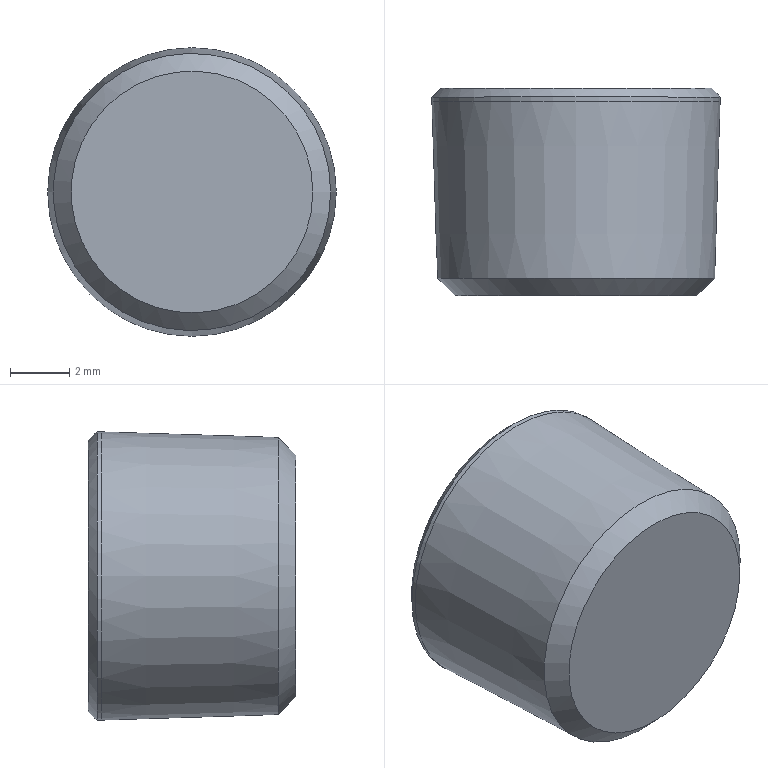Part | STEP file | solid 226 | 1 solid | 13 faces | box 9.737 x 7 x 9.737 mm | volume 407.483 mm3 | plane 9 | cone 4